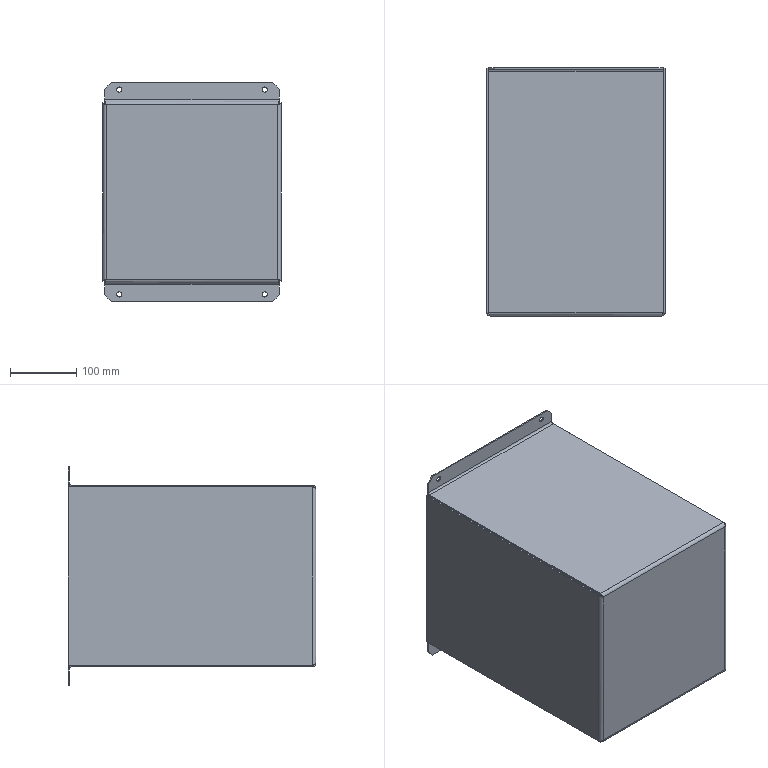Part | STEP file | HXGR200008-05-14 | 1 solid | 73 faces | box 270 x 375 x 331 mm | volume 959853 mm3 | plane 43 | cylinder 22 | spline 8 | commonest cylinder face diameters 8 x8 6 x6 10 x6 60 x2